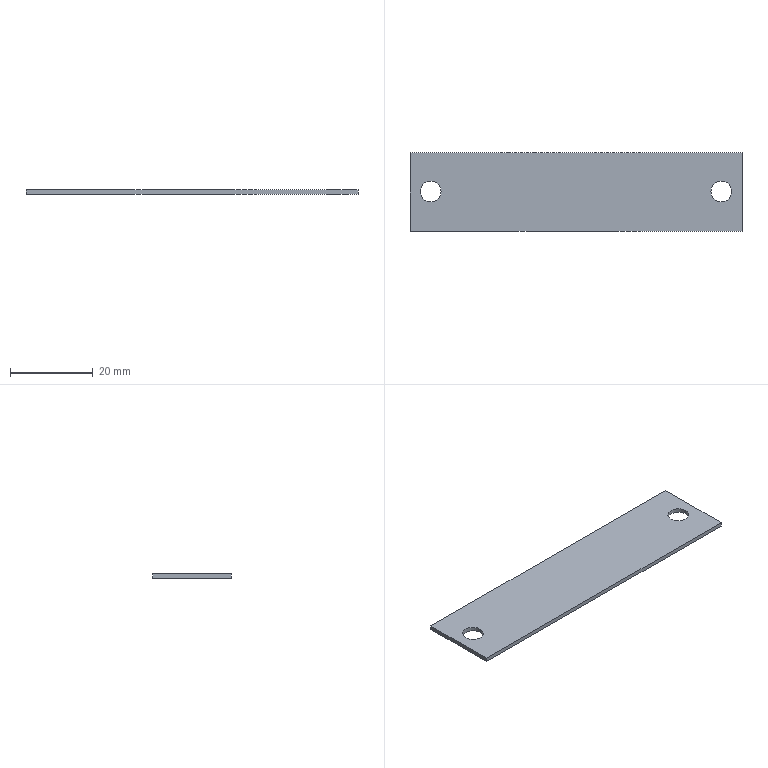Part | SolidWorks | features Extrusion 1, HoleWzd 1 | 1 solid | 10 faces | box 80 x 19 x 1 mm | volume 1481 mm3 | plane 6 | cylinder 4 | commonest cylinder face diameters 5 x4
STEP:
#1=CARTESIAN_POINT('',(-37.5,9.622,0.));
#2=VERTEX_POINT('',#1);
#3=CARTESIAN_POINT('',(-32.5,9.622,0.));
#4=VERTEX_POINT('',#3);
#5=CARTESIAN_POINT('',(-35.,9.622,0.));
#6=DIRECTION('',(0.,0.,1.));
#7=DIRECTION('',(1.,0.,0.));
#8=AXIS2_PLACEMENT_3D('',#5,#6,#7);
#9=CIRCLE('',#8,2.5);
#10=EDGE_CURVE('',#2,#4,#9,.T.);
#11=ORIENTED_EDGE('',*,*,#10,.F.);
#12=CARTESIAN_POINT('',(-37.5,9.622,1.));
#13=VERTEX_POINT('',#12);
#14=CARTESIAN_POINT('',(-37.5,9.622,1.));
#15=DIRECTION('',(0.,0.,1.));
#16=VECTOR('',#15,1000.);
#17=LINE('',#14,#16);
#18=EDGE_CURVE('',#2,#13,#17,.T.);
#19=ORIENTED_EDGE('',*,*,#18,.T.);
#20=CARTESIAN_POINT('',(-32.5,9.622,1.));
#21=VERTEX_POINT('',#20);
#22=CARTESIAN_POINT('',(-35.,9.622,1.));
#23=DIRECTION('',(0.,0.,1.));
#24=DIRECTION('',(1.,0.,0.));
#25=AXIS2_PLACEMENT_3D('',#22,#23,#24);
#26=CIRCLE('',#25,2.5);
#27=EDGE_CURVE('',#13,#21,#26,.T.);
#28=ORIENTED_EDGE('',*,*,#27,.T.);
#29=CARTESIAN_POINT('',(-32.5,9.622,1.));
#30=DIRECTION('',(0.,0.,1.));
#31=VECTOR('',#30,1000.);
#32=LINE('',#29,#31);
#33=EDGE_CURVE('',#4,#21,#32,.T.);
#34=ORIENTED_EDGE('',*,*,#33,.F.);
#35=EDGE_LOOP('',(#11,#19,#28,#34));
#36=FACE_OUTER_BOUND('',#35,.T.);
#37=CARTESIAN_POINT('',(-35.,9.622,1.));
#38=DIRECTION('',(0.,0.,1.));
#39=DIRECTION('',(1.,0.,0.));
#40=AXIS2_PLACEMENT_3D('',#37,#38,#39);
#41=CYLINDRICAL_SURFACE('',#40,2.5);
#42=ADVANCED_FACE('',(#36),#41,.F.);
#43=CARTESIAN_POINT('',(32.5,9.622,0.));
#44=VERTEX_POINT('',#43);
#45=CARTESIAN_POINT('',(37.5,9.622,0.));
#46=VERTEX_POINT('',#45);
#47=CARTESIAN_POINT('',(35.,9.622,0.));
#48=DIRECTION('',(0.,0.,1.));
#49=DIRECTION('',(1.,0.,0.));
#50=AXIS2_PLACEMENT_3D('',#47,#48,#49);
#51=CIRCLE('',#50,2.5);
#52=EDGE_CURVE('',#44,#46,#51,.T.);
#53=ORIENTED_EDGE('',*,*,#52,.F.);
#54=CARTESIAN_POINT('',(32.5,9.622,1.));
#55=VERTEX_POINT('',#54);
#56=CARTESIAN_POINT('',(32.5,9.622,1.));
#57=DIRECTION('',(0.,0.,1.));
#58=VECTOR('',#57,1000.);
#59=LINE('',#56,#58);
#60=EDGE_CURVE('',#44,#55,#59,.T.);
#61=ORIENTED_EDGE('',*,*,#60,.T.);
#62=CARTESIAN_POINT('',(37.5,9.622,1.));
#63=VERTEX_POINT('',#62);
#64=CARTESIAN_POINT('',(35.,9.622,1.));
#65=DIRECTION('',(0.,0.,1.));
#66=DIRECTION('',(1.,0.,0.));
#67=AXIS2_PLACEMENT_3D('',#64,#65,#66);
#68=CIRCLE('',#67,2.5);
#69=EDGE_CURVE('',#55,#63,#68,.T.);
#70=ORIENTED_EDGE('',*,*,#69,.T.);
#71=CARTESIAN_POINT('',(37.5,9.622,1.));
#72=DIRECTION('',(0.,0.,1.));
#73=VECTOR('',#72,1000.);
#74=LINE('',#71,#73);
#75=EDGE_CURVE('',#46,#63,#74,.T.);
#76=ORIENTED_EDGE('',*,*,#75,.F.);
#77=EDGE_LOOP('',(#53,#61,#70,#76));
#78=FACE_OUTER_BOUND('',#77,.T.);
#79=CARTESIAN_POINT('',(35.,9.622,1.));
#80=DIRECTION('',(0.,0.,1.));
#81=DIRECTION('',(1.,0.,0.));
#82=AXIS2_PLACEMENT_3D('',#79,#80,#81);
#83=CYLINDRICAL_SURFACE('',#82,2.5);
#84=ADVANCED_FACE('',(#78),#83,.F.);
#85=CARTESIAN_POINT('',(-40.,19.,0.));
#86=VERTEX_POINT('',#85);
#87=CARTESIAN_POINT('',(-40.,0.,0.));
#88=VERTEX_POINT('',#87);
#89=CARTESIAN_POINT('',(-40.,19.,0.));
#90=DIRECTION('',(0.,-1.,0.));
#91=VECTOR('',#90,1000.);
#92=LINE('',#89,#91);
#93=EDGE_CURVE('',#86,#88,#92,.T.);
#94=ORIENTED_EDGE('',*,*,#93,.T.);
#95=CARTESIAN_POINT('',(-40.,0.,1.));
#96=VERTEX_POINT('',#95);
#97=CARTESIAN_POINT('',(-40.,0.,1.));
#98=DIRECTION('',(0.,0.,-1.));
#99=VECTOR('',#98,1000.);
#100=LINE('',#97,#99);
#101=EDGE_CURVE('',#96,#88,#100,.T.);
#102=ORIENTED_EDGE('',*,*,#101,.F.);
#103=CARTESIAN_POINT('',(-40.,19.,1.));
#104=VERTEX_POINT('',#103);
#105=CARTESIAN_POINT('',(-40.,19.,1.));
#106=DIRECTION('',(0.,-1.,0.));
#107=VECTOR('',#106,1000.);
#108=LINE('',#105,#107);
#109=EDGE_CURVE('',#104,#96,#108,.T.);
#110=ORIENTED_EDGE('',*,*,#109,.F.);
#111=CARTESIAN_POINT('',(-40.,19.,1.));
#112=DIRECTION('',(0.,0.,-1.));
#113=VECTOR('',#112,1000.);
#114=LINE('',#111,#113);
#115=EDGE_CURVE('',#104,#86,#114,.T.);
#116=ORIENTED_EDGE('',*,*,#115,.T.);
#117=EDGE_LOOP('',(#94,#102,#110,#116));
#118=FACE_OUTER_BOUND('',#117,.T.);
#119=CARTESIAN_POINT('',(-40.,19.,1.));
#120=DIRECTION('',(1.,0.,0.));
#121=DIRECTION('',(0.,1.,0.));
#122=AXIS2_PLACEMENT_3D('',#119,#120,#121);
#123=PLANE('',#122);
#124=ADVANCED_FACE('',(#118),#123,.F.);
#125=CARTESIAN_POINT('',(40.,0.,0.));
#126=VERTEX_POINT('',#125);
#127=CARTESIAN_POINT('',(-40.,0.,0.));
#128=DIRECTION('',(1.,0.,0.));
#129=VECTOR('',#128,1000.);
#130=LINE('',#127,#129);
#131=EDGE_CURVE('',#88,#126,#130,.T.);
#132=ORIENTED_EDGE('',*,*,#131,.T.);
#133=CARTESIAN_POINT('',(40.,0.,1.));
#134=VERTEX_POINT('',#133);
#135=CARTESIAN_POINT('',(40.,0.,1.));
#136=DIRECTION('',(0.,0.,-1.));
#137=VECTOR('',#136,1000.);
#138=LINE('',#135,#137);
#139=EDGE_CURVE('',#134,#126,#138,.T.);
#140=ORIENTED_EDGE('',*,*,#139,.F.);
#141=CARTESIAN_POINT('',(-40.,0.,1.));
#142=DIRECTION('',(1.,0.,0.));
#143=VECTOR('',#142,1000.);
#144=LINE('',#141,#143);
#145=EDGE_CURVE('',#96,#134,#144,.T.);
#146=ORIENTED_EDGE('',*,*,#145,.F.);
#147=ORIENTED_EDGE('',*,*,#101,.T.);
#148=EDGE_LOOP('',(#132,#140,#146,#147));
#149=FACE_OUTER_BOUND('',#148,.T.);
#150=CARTESIAN_POINT('',(-40.,0.,1.));
#151=DIRECTION('',(0.,1.,0.));
#152=DIRECTION('',(0.,0.,1.));
#153=AXIS2_PLACEMENT_3D('',#150,#151,#152);
#154=PLANE('',#153);
#155=ADVANCED_FACE('',(#149),#154,.F.);
#156=CARTESIAN_POINT('',(40.,19.,0.));
#157=VERTEX_POINT('',#156);
#158=CARTESIAN_POINT('',(40.,19.,0.));
#159=DIRECTION('',(0.,1.,0.));
#160=VECTOR('',#159,1000.);
#161=LINE('',#158,#160);
#162=EDGE_CURVE('',#126,#157,#161,.T.);
#163=ORIENTED_EDGE('',*,*,#162,.T.);
#164=CARTESIAN_POINT('',(40.,19.,1.));
#165=VERTEX_POINT('',#164);
#166=CARTESIAN_POINT('',(40.,19.,1.));
#167=DIRECTION('',(0.,0.,-1.));
#168=VECTOR('',#167,1000.);
#169=LINE('',#166,#168);
#170=EDGE_CURVE('',#165,#157,#169,.T.);
#171=ORIENTED_EDGE('',*,*,#170,.F.);
#172=CARTESIAN_POINT('',(40.,19.,1.));
#173=DIRECTION('',(0.,1.,0.));
#174=VECTOR('',#173,1000.);
#175=LINE('',#172,#174);
#176=EDGE_CURVE('',#134,#165,#175,.T.);
#177=ORIENTED_EDGE('',*,*,#176,.F.);
#178=ORIENTED_EDGE('',*,*,#139,.T.);
#179=EDGE_LOOP('',(#163,#171,#177,#178));
#180=FACE_OUTER_BOUND('',#179,.T.);
#181=CARTESIAN_POINT('',(40.,19.,1.));
#182=DIRECTION('',(-1.,0.,0.));
#183=DIRECTION('',(0.,-1.,0.));
#184=AXIS2_PLACEMENT_3D('',#181,#182,#183);
#185=PLANE('',#184);
#186=ADVANCED_FACE('',(#180),#185,.F.);
#187=CARTESIAN_POINT('',(-40.,19.,0.));
#188=DIRECTION('',(-1.,0.,0.));
#189=VECTOR('',#188,1000.);
#190=LINE('',#187,#189);
#191=EDGE_CURVE('',#157,#86,#190,.T.);
#192=ORIENTED_EDGE('',*,*,#191,.T.);
#193=ORIENTED_EDGE('',*,*,#115,.F.);
#194=CARTESIAN_POINT('',(-40.,19.,1.));
#195=DIRECTION('',(-1.,0.,0.));
#196=VECTOR('',#195,1000.);
#197=LINE('',#194,#196);
#198=EDGE_CURVE('',#165,#104,#197,.T.);
#199=ORIENTED_EDGE('',*,*,#198,.F.);
#200=ORIENTED_EDGE('',*,*,#170,.T.);
#201=EDGE_LOOP('',(#192,#193,#199,#200));
#202=FACE_OUTER_BOUND('',#201,.T.);
#203=CARTESIAN_POINT('',(-40.,19.,1.));
#204=DIRECTION('',(0.,-1.,0.));
#205=DIRECTION('',(0.,0.,-1.));
#206=AXIS2_PLACEMENT_3D('',#203,#204,#205);
#207=PLANE('',#206);
#208=ADVANCED_FACE('',(#202),#207,.F.);
#209=CARTESIAN_POINT('',(-35.,9.622,1.));
#210=DIRECTION('',(0.,0.,1.));
#211=DIRECTION('',(1.,0.,0.));
#212=AXIS2_PLACEMENT_3D('',#209,#210,#211);
#213=CIRCLE('',#212,2.5);
#214=EDGE_CURVE('',#21,#13,#213,.T.);
#215=ORIENTED_EDGE('',*,*,#214,.F.);
#216=ORIENTED_EDGE('',*,*,#27,.F.);
#217=EDGE_LOOP('',(#215,#216));
#218=FACE_BOUND('',#217,.T.);
#219=CARTESIAN_POINT('',(35.,9.622,1.));
#220=DIRECTION('',(0.,0.,1.));
#221=DIRECTION('',(1.,0.,0.));
#222=AXIS2_PLACEMENT_3D('',#219,#220,#221);
#223=CIRCLE('',#222,2.5);
#224=EDGE_CURVE('',#63,#55,#223,.T.);
#225=ORIENTED_EDGE('',*,*,#224,.F.);
#226=ORIENTED_EDGE('',*,*,#69,.F.);
#227=EDGE_LOOP('',(#225,#226));
#228=FACE_BOUND('',#227,.T.);
#229=ORIENTED_EDGE('',*,*,#109,.T.);
#230=ORIENTED_EDGE('',*,*,#145,.T.);
#231=ORIENTED_EDGE('',*,*,#176,.T.);
#232=ORIENTED_EDGE('',*,*,#198,.T.);
#233=EDGE_LOOP('',(#229,#230,#231,#232));
#234=FACE_OUTER_BOUND('',#233,.T.);
#235=CARTESIAN_POINT('',(0.,0.,1.));
#236=DIRECTION('',(0.,0.,1.));
#237=DIRECTION('',(1.,0.,0.));
#238=AXIS2_PLACEMENT_3D('',#235,#236,#237);
#239=PLANE('',#238);
#240=ADVANCED_FACE('',(#218,#228,#234),#239,.T.);
#241=CARTESIAN_POINT('',(-35.,9.622,0.));
#242=DIRECTION('',(0.,0.,1.));
#243=DIRECTION('',(1.,0.,0.));
#244=AXIS2_PLACEMENT_3D('',#241,#242,#243);
#245=CIRCLE('',#244,2.5);
#246=EDGE_CURVE('',#4,#2,#245,.T.);
#247=ORIENTED_EDGE('',*,*,#246,.T.);
#248=ORIENTED_EDGE('',*,*,#10,.T.);
#249=EDGE_LOOP('',(#247,#248));
#250=FACE_BOUND('',#249,.T.);
#251=CARTESIAN_POINT('',(35.,9.622,0.));
#252=DIRECTION('',(0.,0.,1.));
#253=DIRECTION('',(1.,0.,0.));
#254=AXIS2_PLACEMENT_3D('',#251,#252,#253);
#255=CIRCLE('',#254,2.5);
#256=EDGE_CURVE('',#46,#44,#255,.T.);
#257=ORIENTED_EDGE('',*,*,#256,.T.);
#258=ORIENTED_EDGE('',*,*,#52,.T.);
#259=EDGE_LOOP('',(#257,#258));
#260=FACE_BOUND('',#259,.T.);
#261=ORIENTED_EDGE('',*,*,#93,.F.);
#262=ORIENTED_EDGE('',*,*,#191,.F.);
#263=ORIENTED_EDGE('',*,*,#162,.F.);
#264=ORIENTED_EDGE('',*,*,#131,.F.);
#265=EDGE_LOOP('',(#261,#262,#263,#264));
#266=FACE_OUTER_BOUND('',#265,.T.);
#267=CARTESIAN_POINT('',(0.,0.,0.));
#268=DIRECTION('',(0.,0.,1.));
#269=DIRECTION('',(1.,0.,0.));
#270=AXIS2_PLACEMENT_3D('',#267,#268,#269);
#271=PLANE('',#270);
#272=ADVANCED_FACE('',(#250,#260,#266),#271,.F.);
#273=ORIENTED_EDGE('',*,*,#60,.F.);
#274=ORIENTED_EDGE('',*,*,#256,.F.);
#275=ORIENTED_EDGE('',*,*,#75,.T.);
#276=ORIENTED_EDGE('',*,*,#224,.T.);
#277=EDGE_LOOP('',(#273,#274,#275,#276));
#278=FACE_OUTER_BOUND('',#277,.T.);
#279=CARTESIAN_POINT('',(35.,9.622,1.));
#280=DIRECTION('',(0.,0.,1.));
#281=DIRECTION('',(1.,0.,0.));
#282=AXIS2_PLACEMENT_3D('',#279,#280,#281);
#283=CYLINDRICAL_SURFACE('',#282,2.5);
#284=ADVANCED_FACE('',(#278),#283,.F.);
#285=ORIENTED_EDGE('',*,*,#18,.F.);
#286=ORIENTED_EDGE('',*,*,#246,.F.);
#287=ORIENTED_EDGE('',*,*,#33,.T.);
#288=ORIENTED_EDGE('',*,*,#214,.T.);
#289=EDGE_LOOP('',(#285,#286,#287,#288));
#290=FACE_OUTER_BOUND('',#289,.T.);
#291=CARTESIAN_POINT('',(-35.,9.622,1.));
#292=DIRECTION('',(0.,0.,1.));
#293=DIRECTION('',(1.,0.,0.));
#294=AXIS2_PLACEMENT_3D('',#291,#292,#293);
#295=CYLINDRICAL_SURFACE('',#294,2.5);
#296=ADVANCED_FACE('',(#290),#295,.F.);
#297=CLOSED_SHELL('',(#42,#84,#124,#155,#186,#208,#240,#272,#284,#296));
#298=MANIFOLD_SOLID_BREP('',#297);
#299=CARTESIAN_POINT('',(0.,0.,0.));
#300=DIRECTION('',(0.,0.,1.));
#301=DIRECTION('',(1.,0.,0.));
#302=AXIS2_PLACEMENT_3D('',#299,#300,#301);
#303=(LENGTH_UNIT()NAMED_UNIT(*)SI_UNIT(.MILLI.,.METRE.));
#304=UNCERTAINTY_MEASURE_WITH_UNIT(LENGTH_MEASURE(0.00001),#303,'','');
#305=(NAMED_UNIT(*)PLANE_ANGLE_UNIT()SI_UNIT($,.RADIAN.));
#306=(NAMED_UNIT(*)SI_UNIT($,.STERADIAN.)SOLID_ANGLE_UNIT());
#307=(GEOMETRIC_REPRESENTATION_CONTEXT(3)GLOBAL_UNCERTAINTY_ASSIGNED_CONTEXT((#304))GLOBAL_UNIT_ASSIGNED_CONTEXT((#303,#305,#306))REPRESENTATION_CONTEXT('',''));
#308=ADVANCED_BREP_SHAPE_REPRESENTATION('',(#298,#302),#307);